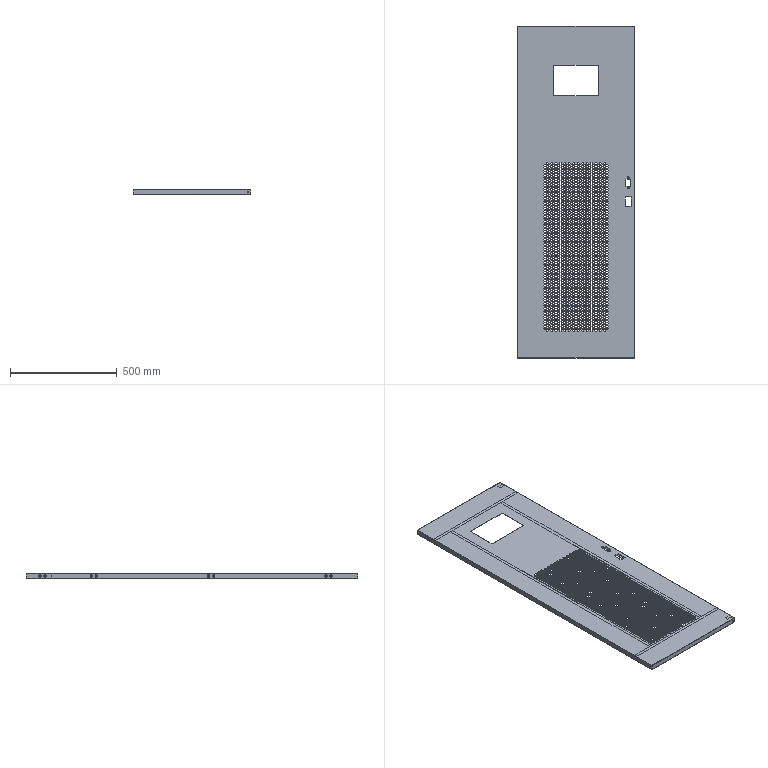Part | SolidWorks | features MirrorCompFeat 1, ReferencePattern 1 | 7 solids | 11640 faces | volume 1107587 mm3 | plane 11532 | cylinder 92 | spline 16 | commonest cylinder face diameters 5.5 x16 6.5 x16 11.5 x16 0.2 x14 4.5 x12 2.6 x8